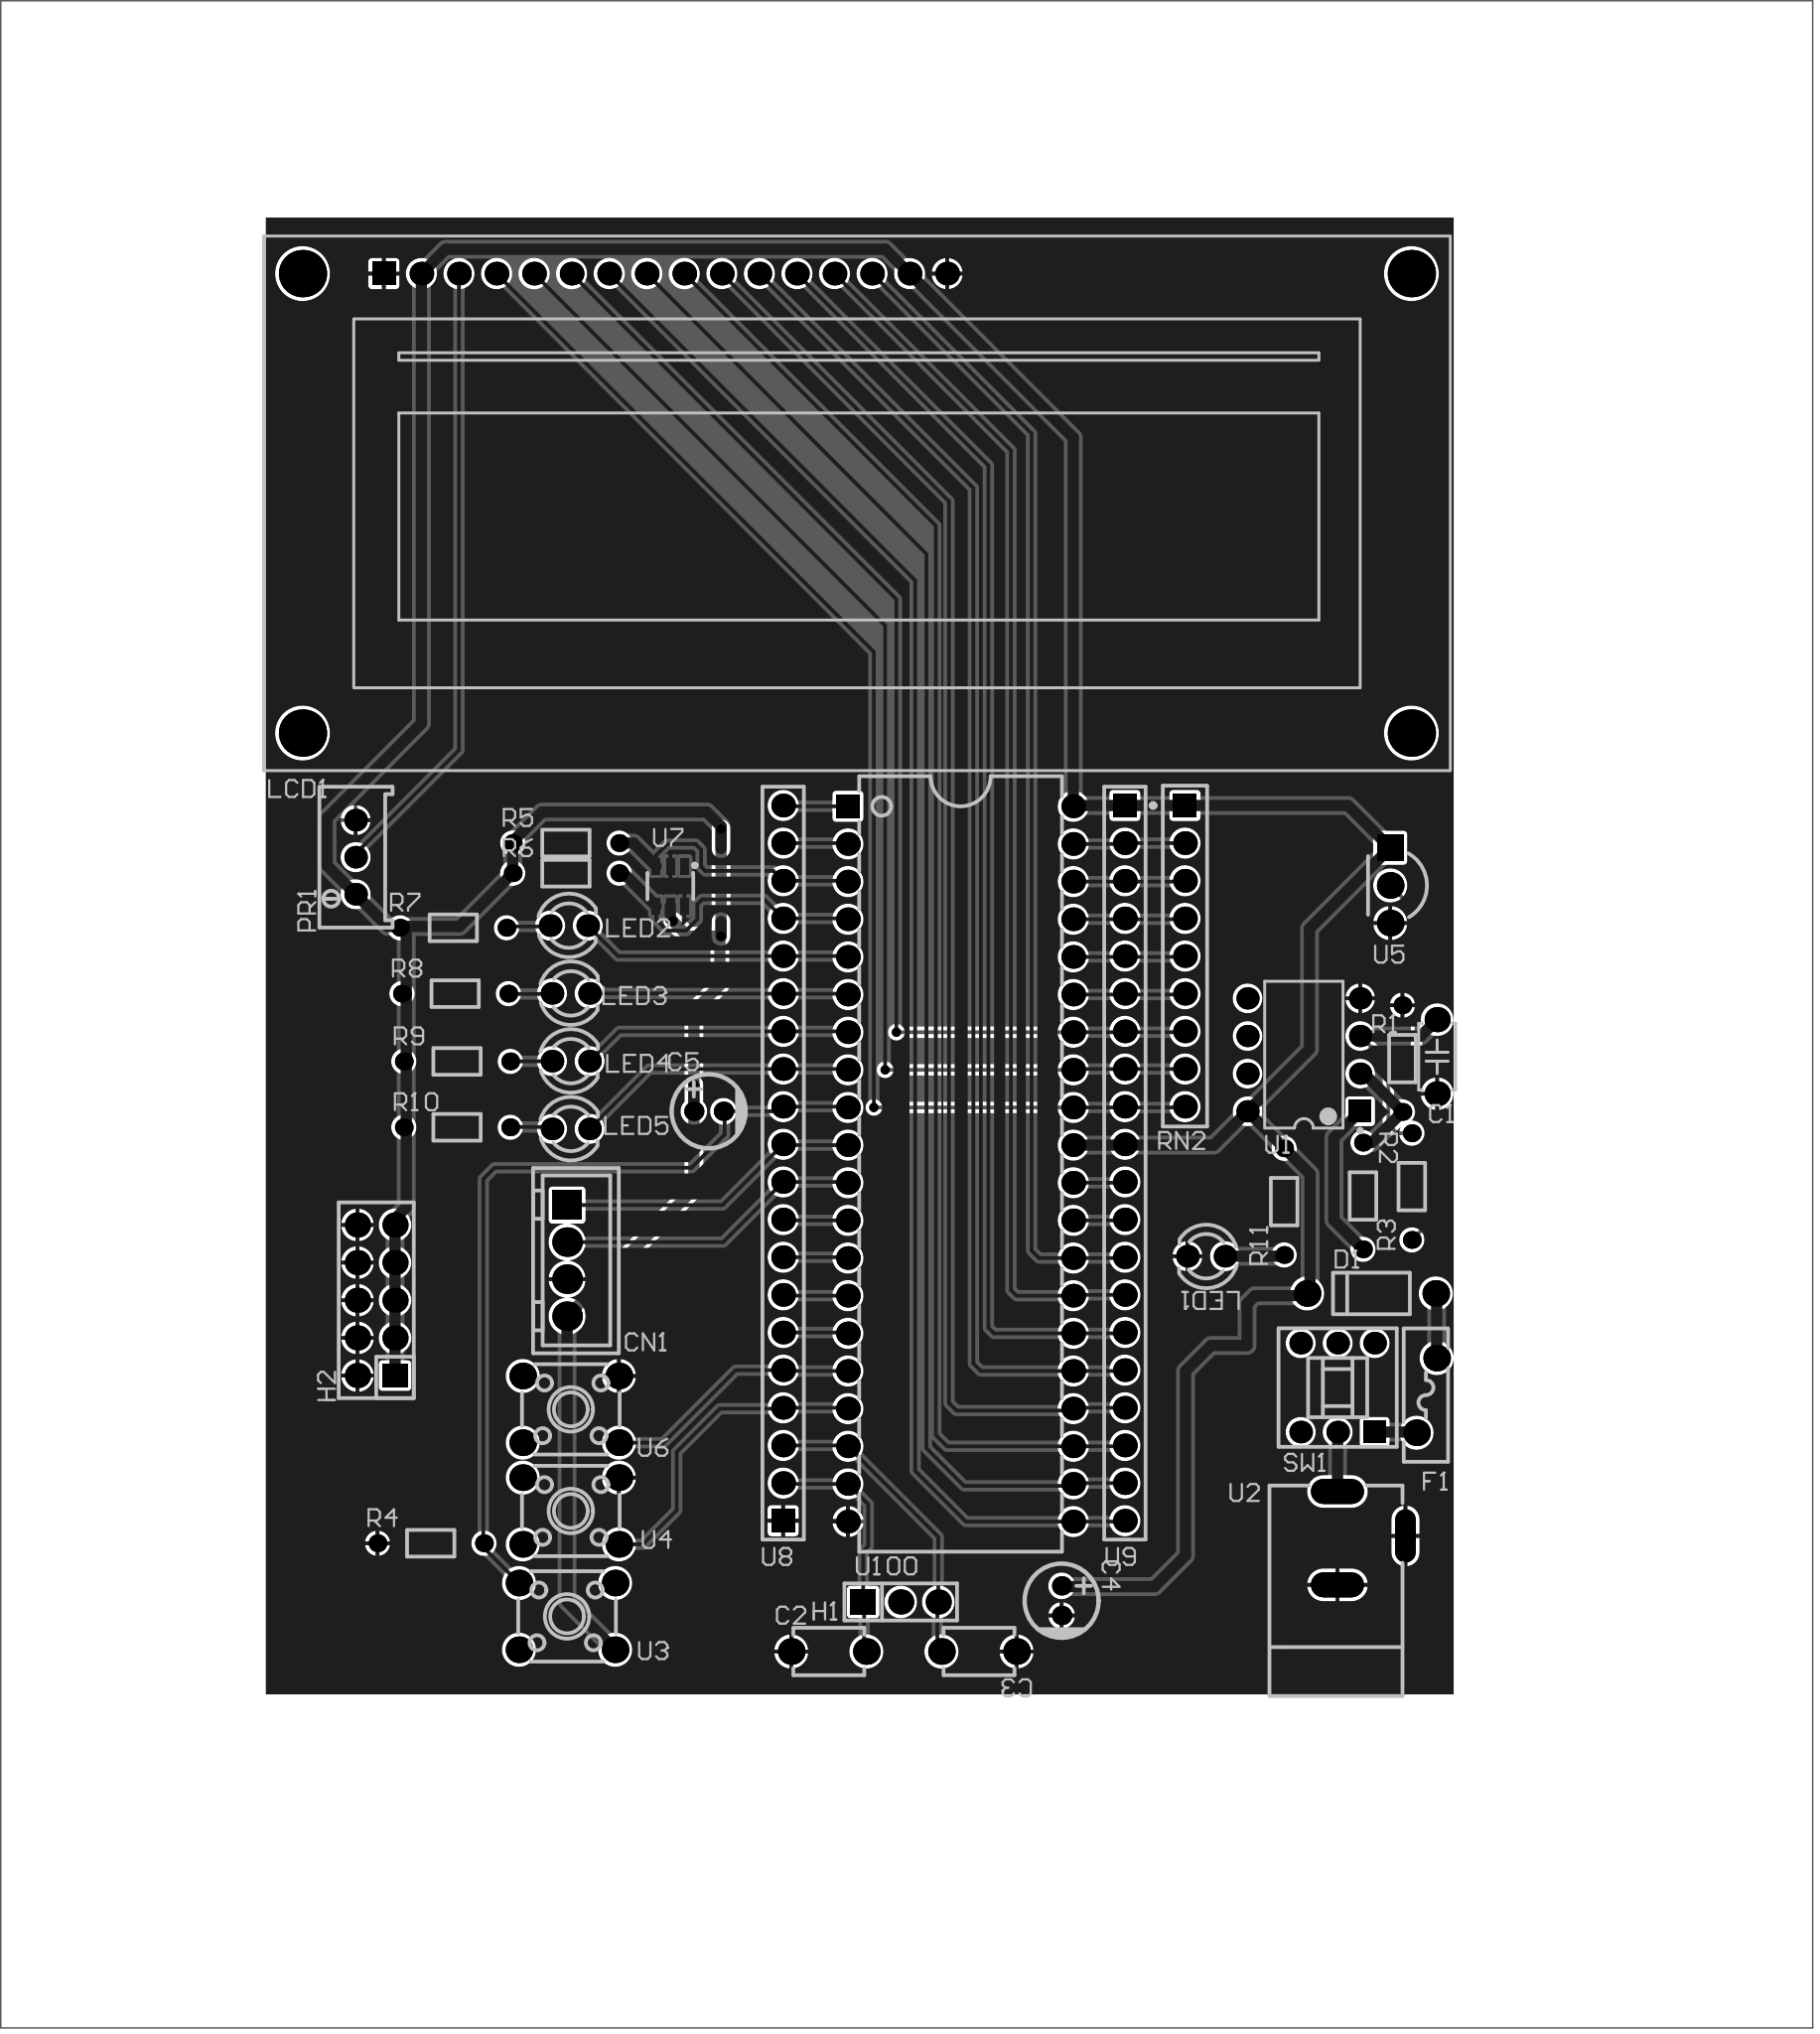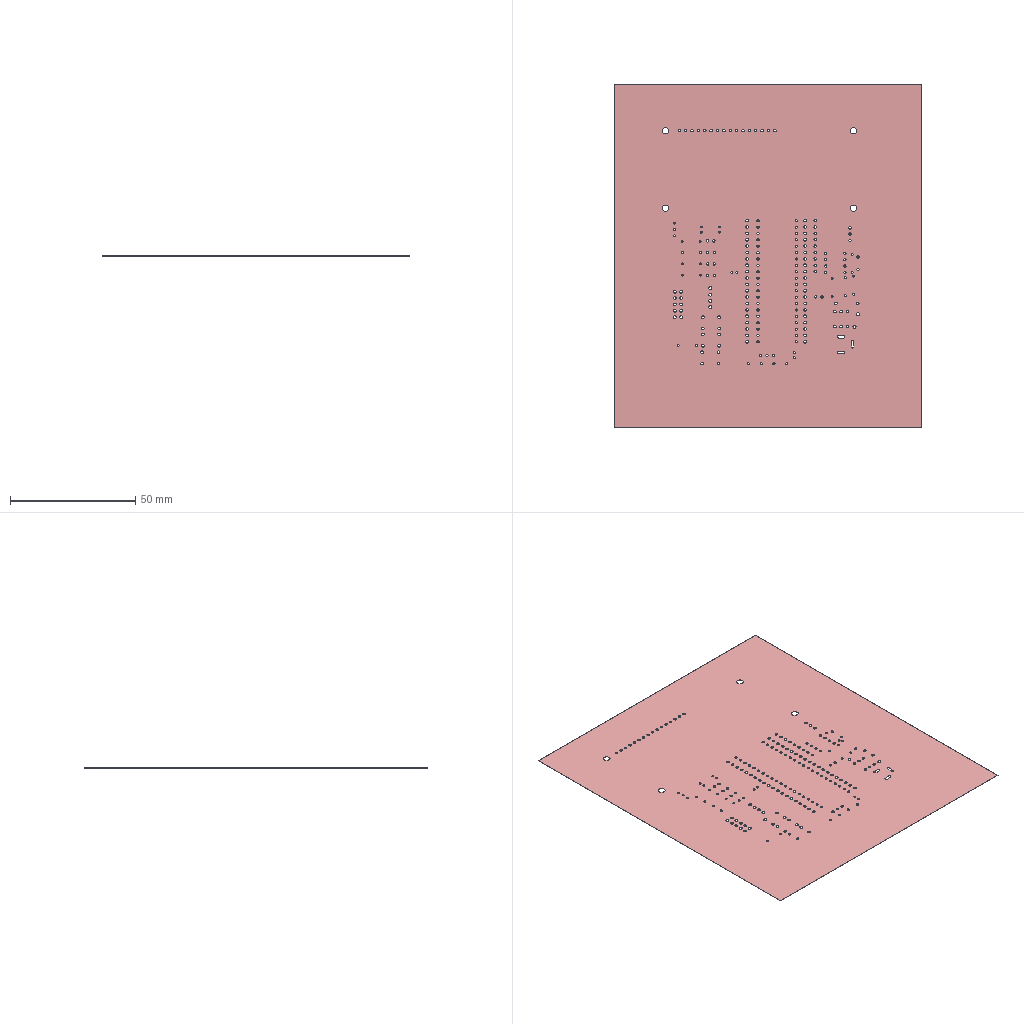Circuit board layout | Altium Designer | box 122.6 x 136.8 x 0.1 mm
Layer stack:
# Altium Designer layer stack of  (unit mm; dielectric type: 0 none, 1 core, 2 prepreg, 3 surface material)
index,name,kind,layer,copper_thickness_mm,dielectric_type,dielectric_thickness_mm,dielectric_material,dielectric_constant
0,Top Paste Mask Layer,other,,,,,,
1,Top Silkscreen Layer,other,,,,,,
2,Top Solder Mask Layer,dielectric,,,3,0.01,,3.3
3,Top Layer,copper,Top Layer,0.035,,,,
4,Bottom Layer,copper,Bottom Layer,0.035,,,,
5,Bottom Solder Mask Layer,dielectric,,,3,0.01,,3.3
6,Bottom Silkscreen Layer,other,,,,,,
7,Bottom Paste Mask Layer,other,,,,,,
# drill layer pairs: low layer,high layer
drill_pair,Top Layer,Bottom Layer
Part placement:
Designator,Comment,Layer,Footprint,Center-X(mm),Center-Y(mm),Rotation
CN1,HEADER 4,TopLayer,CONN-TH_XH-4A,108.154,121.621,270
D1,1N4007,TopLayer,DO-41_BD2.4-L4.7-P8.70-D0.9-RD,162.561,119.407,0
F1,JK60-050,TopLayer,FUSE-TH_L8.9-W3.0-P5.10-D0.6-S1.20,166.29,112.529,90
H1,PZ254V-11-03P_C2937625,TopLayer,HDR-TH_3P-P2.54-V-M_PZ254V-11-03P,130.722,98.593,0
LCD1,HS1602A,TopLayer,LCD1602,127.762,172.72,0
LED2,HL-304S9AD,TopLayer,LED-TH_BD3.0-P2.54-FD,108.281,144.227,0
LED3,HL-304S9AD,TopLayer,LED-TH_BD3.0-P2.54-FD,108.408,139.655,0
LED4,HL-304S9AD,TopLayer,LED-TH_BD3.0-P2.54-FD,108.408,135.083,0
LED5,HL-304S9AD,TopLayer,LED-TH_BD3.0-P2.54-FD,108.408,130.511,0
RN2,10K,TopLayer,RES-ARRAY-TH_9P-P2.54-D1.0,149.948,142.172,270
SW1,HX 8-8 ZS,TopLayer,SW-TH_6P-L8.0-W8.0-P2.50-TL,160.275,113.057,180
U2,DC005-2.5,TopLayer,DC-IN-TH_DC005-2.5MM,162.561,102.897,90
U3,TC-00104FS-075E,TopLayer,KEY-TH_4P-L6.0-W6.0-P4.50-LS6.5,108.154,97.618,0
U4,TC-00104FS-075E,TopLayer,KEY-TH_4P-L6.0-W6.0-P4.50-LS6.5,108.408,104.73,180
U6,TC-00104FS-075E,TopLayer,KEY-TH_4P-L6.0-W6.0-P4.50-LS6.5,108.408,111.588,180
U5,LM35DZ/NOPB,TopLayer,TO-92-3_L4.8-W3.7-P2.54-L,163.83,146.939,270
U7,ADS1110A1IDBVR,TopLayer,SOT-23-6_L2.9-W1.6-P0.95-LS2.8-BR,115.139,146.894,90
U8,[Plugin] 2.54MM 1*20P straight female header-H5.0,TopLayer,HDR-TH_20P-P2.54_C9900009338,122.77,128.202,90
U9,[Plugin] 2.54MM 1*20P straight female header-H5.0,TopLayer,HDR-TH_20P-P2.54_C9900009338,145.884,128.202,270
U100,STC89C52RC-40I,TopLayer,DIP-40_L52.0-W13.7-P2.54-LS15.2-BL,134.771,128.147,270
U1,LM358AN,TopLayer,DIP-8_L9.8-W6.6-P2.54-LS7.6-BL,157.988,135.509,90
C1,10nF,TopLayer,CAP-TH_L4.5-W2.5-P5.00-D0.5,167.005,135.382,90
H2,,TopLayer,HDR-TH_10P-P2.54-V-F-R2-C5-S2.54,95.248,118.95,90
PR1,10kΩ,TopLayer,R_3296,93.853,148.844,90
R1,10kΩ,TopLayer,Res_1/8W,164.655,135.255,270
R2,10kΩ,TopLayer,Res_1/8W,161.988,125.984,270
R3,10kΩ,TopLayer,Res_1/8W,165.291,126.619,90
C2,22pF,TopLayer,CAP-TH_L4.8-W3.2-P5.08-D0.5,125.857,95.25,0
C3,22pF,TopLayer,CAP-TH_L4.8-W3.2-P5.08-D0.5,136.017,95.25,180
C4,10uF,TopLayer,CAP-TH_BD5.0-P2.00-D0.8-FD-10UF50VC110GL,141.605,98.679,270
C5,10uF,TopLayer,CAP-TH_BD5.0-P2.00-D0.8-FD-10UF50VC110GL,117.729,131.699,0
R4,10kΩ,TopLayer,Res_1/8W,98.933,102.552,0
R5,10kΩ,TopLayer,Res_1/8W,108.077,149.796,0
R6,10kΩ,TopLayer,Res_1/8W,108.077,147.764,0
R7,1kΩ,TopLayer,Res_1/8W,100.457,144.081,0
R8,1kΩ,TopLayer,Res_1/8W,100.584,139.636,0
R9,1kΩ,TopLayer,Res_1/8W,100.711,135.064,0
R10,1kΩ,TopLayer,Res_1/8W,100.711,130.619,0
LED1,,TopLayer,LED_TH-3mm,151.384,121.92,180
R11,1kΩ,TopLayer,Res_1/8W,156.655,125.603,90
Pad and via stacks:
# Altium Designer via and pad stacks of  (unit mm). Each distinct definition once, with the count of objects using it.
# via: kind,start_layer,end_layer,hole_mm,diameter_mm,mode(0 simple;1 top-mid-bottom;2 full stack),diameter_per_layer,count,example_net
# pad: kind,layer,hole_mm,hole_type(0 round;1 square;2 slot),plating,top_size,top_shape(1 round;2 rect;3 octagon;9 rounded rect),mid_size,bottom_size,mode,footprint,size_per_layer,count,example
pad,Multi-Layer,1.2,0,plated,2x2,1,2x2,2x2,0,CONN-TH_XH-4A,,3,CN1.4
pad,Multi-Layer,1.2,0,plated,2x2,2,2x2,2x2,0,CONN-TH_XH-4A,,1,CN1.1
pad,Multi-Layer,1,0,plated,1.8x1.8,1,1.8x1.8,1.8x1.8,0,DO-41_BD2.4-L4.7-P8.70-D0.9-RD,,2,D1.1
pad,Multi-Layer,1.2,0,plated,1.8x1.8,1,1.8x1.8,1.8x1.8,0,FUSE-TH_L8.9-W3.0-P5.10-D0.6-S1.20,,2,F1.1
pad,Multi-Layer,1.02,0,plated,1.7x1.7,2,1.7x1.7,1.7x1.7,0,HDR-TH_3P-P2.54-V-M_PZ254V-11-03P,,1,H1.1
pad,Multi-Layer,1.02,0,plated,1.7x1.7,1,1.7x1.7,1.7x1.7,0,HDR-TH_3P-P2.54-V-M_PZ254V-11-03P,,2,H1.2
pad,Multi-Layer,1,0,plated,1.6x1.6,1,1.6x1.6,1.6x1.6,0,LCD1602,,15,LCD1.16
pad,Multi-Layer,1,0,plated,1.6x1.6,2,1.6x1.6,1.6x1.6,0,LCD1602,,1,LCD1.1
pad,Multi-Layer,2.5,2,plated,3.2x3.2,1,3.2x3.2,3.2x3.2,0,LCD1602,,4,LCD1.0
pad,Multi-Layer,0.9144,0,plated,1.524x1.524,1,1.524x1.524,1.524x1.524,0,LED-TH_BD3.0-P2.54-FD,,8,LED2.1
pad,Multi-Layer,1,0,plated,1.6x1.6,2,1.6x1.6,1.6x1.6,0,RES-ARRAY-TH_9P-P2.54-D1.0,,1,RN2.1
pad,Multi-Layer,1,0,plated,1.6x1.6,1,1.6x1.6,1.6x1.6,0,RES-ARRAY-TH_9P-P2.54-D1.0,,8,RN2.2
pad,Multi-Layer,1,0,plated,1.524x1.524,1,1.524x1.524,1.524x1.524,0,SW-TH_6P-L8.0-W8.0-P2.50-TL,,5,SW1.4
pad,Multi-Layer,1,0,plated,1.524x1.524,2,1.524x1.524,1.524x1.524,0,SW-TH_6P-L8.0-W8.0-P2.50-TL,,1,SW1.1
pad,Multi-Layer,1,2,plated,1.7x3.6,1,1.7x3.6,1.7x3.6,0,DC-IN-TH_DC005-2.5MM,,2,U2.3
pad,Multi-Layer,0.8,2,plated,1.4x3.6,1,1.4x3.6,1.4x3.6,0,DC-IN-TH_DC005-2.5MM,,1,U2.2
pad,Multi-Layer,1.1,0,plated,1.8x1.8,1,1.8x1.8,1.8x1.8,0,KEY-TH_4P-L6.0-W6.0-P4.50-LS6.5,,12,U3.4
pad,Multi-Layer,1,0,plated,1.8x1.8,1,1.8x1.8,1.8x1.8,0,TO-92-3_L4.8-W3.7-P2.54-L,,2,U5.3
pad,Multi-Layer,1,0,plated,1.8x1.8,2,1.8x1.8,1.8x1.8,0,TO-92-3_L4.8-W3.7-P2.54-L,,1,U5.1
pad,Multi-Layer,1.05,0,plated,1.6x1.6,2,1.6x1.6,1.6x1.6,0,HDR-TH_20P-P2.54_C9900009338,,2,U8.1
pad,Multi-Layer,1.05,0,plated,1.6x1.6,1,1.6x1.6,1.6x1.6,0,HDR-TH_20P-P2.54_C9900009338,,38,U8.2
pad,Multi-Layer,0.889,0,plated,1.6x1.6,1,1.6x1.6,1.6x1.6,0,DIP-40_L52.0-W13.7-P2.54-LS15.2-BL,,39,U100.31
pad,Multi-Layer,0.889,0,plated,1.6x1.6,2,1.6x1.6,1.6x1.6,0,DIP-40_L52.0-W13.7-P2.54-LS15.2-BL,,1,U100.1
pad,Multi-Layer,0.9,0,plated,1.5x1.5,2,1.5x1.5,1.5x1.5,0,DIP-8_L9.8-W6.6-P2.54-LS7.6-BL,,1,U1.1
pad,Multi-Layer,0.9,0,plated,1.5x1.5,1,1.5x1.5,1.5x1.5,0,DIP-8_L9.8-W6.6-P2.54-LS7.6-BL,,7,U1.2
pad,Multi-Layer,0.9,0,plated,1.7x1.7,1,1.7x1.7,1.7x1.7,0,CAP-TH_L4.5-W2.5-P5.00-D0.5,,2,C1.2
pad,Multi-Layer,1.1,0,plated,1.7x1.7,1,1.7x1.7,1.7x1.7,0,HDR-TH_10P-P2.54-V-F-R2-C5-S2.54,,9,H2.10
pad,Multi-Layer,1.1,0,plated,1.575x1.7,2,1.575x1.7,1.575x1.7,0,HDR-TH_10P-P2.54-V-F-R2-C5-S2.54,,1,H2.1
pad,Multi-Layer,0.762,0,plated,1.524x1.524,1,1.524x1.524,1.524x1.524,0,R_3296,,3,PR1.2
pad,Multi-Layer,0.8001,0,plated,1.199x1.199,1,1.199x1.199,1.199x1.199,0,Res_1/8W,,22,R1.1
pad,Multi-Layer,0.9,0,plated,1.8x1.8,1,1.8x1.8,1.8x1.8,0,CAP-TH_L4.8-W3.2-P5.08-D0.5,,4,C2.1
pad,Multi-Layer,0.8,0,plated,1.3x1.3,1,1.3x1.3,1.3x1.3,0,CAP-TH_BD5.0-P2.00-D0.8-FD-10UF50VC110GL,,4,C4.1
pad,Multi-Layer,0.9144,0,plated,1.524x1.524,1,1.524x1.524,1.524x1.524,0,LED_TH-3mm,,2,LED1.1
pad,Top Layer,0,0,plated,1.1x0.6,2,1.1x0.6,1.1x0.6,0,SOT-23-6_L2.9-W1.6-P0.95-LS2.8-BR,,6,U7.3
via,Top Layer,Bottom Layer,0.3099,0.62,0,,7,P0.5
Copper pours:
name,layer,net,type(0 solid;1 hatched;2 none)
Top Layer-GND,Top Layer,GND,0
Bottom Layer-GND,Bottom Layer,GND,0
Bottom Layer-GND 1,Bottom Layer,GND,0
Bottom Layer-GND 2,Bottom Layer,GND,0
Design rules, without the lines most boards share:
# Altium Designer design rules of  (exported by Altium Designer, unit mm)
# columns: name | kind | enabled | priority | scope1 | scope2 | descriptor | typed fields (field=value)
Default | 0 | enabled | 1 | All | All | Clearance Constraint (Gap=6mil) (All),(All) | gap=0.1524
Default_1 | 63 | enabled | 1 | All | All | Board Clearance Constraint (Gap=0mil) (All) |
otherClearance | 52 | enabled | 1 | All | All | Hole To Hole Clearance (Gap=11.8mil) (All),(All) | gap=0.2997
Default_2 | 2 | enabled | 1 | All | All | Width Constraint (Min=10mil) (Max=1000mil) (Preferred=10mil) (All) |
differentialPair | 51 | enabled | 1 | All | All | Differential Pairs Uncoupled Length using the Gap Constraints (Min=5mil) (Max=6mil) (Prefered=6mil)  and Width Constraints (Min=5mil) (Max=100mil) (Prefered=100mil) (All) |
Default_3 | 11 | enabled | 1 | All | All | Routing Via (MinHoleWidth=12mil) (MaxHoleWidth=1181mil) (PreferredHoleWidth=12mil) (MinWidth=24mil) (MaxWidth=1969mil) (PreferedWidth=24mil) (All) | via_min_hole=0.3048 via_max_hole=29.997 via_preferred_diameter=0.6096 via_preferred_hole=0.3048
Common | 13 | enabled | 2 | All | All | Solder Mask Expansion (Expansion =2mil) (All) | expansion=0.0508
Common_1 | 13 | enabled | 1 | IsVia | All | Solder Mask Expansion (Expansion =-1000mil) (IsVia) | expansion=-25.4